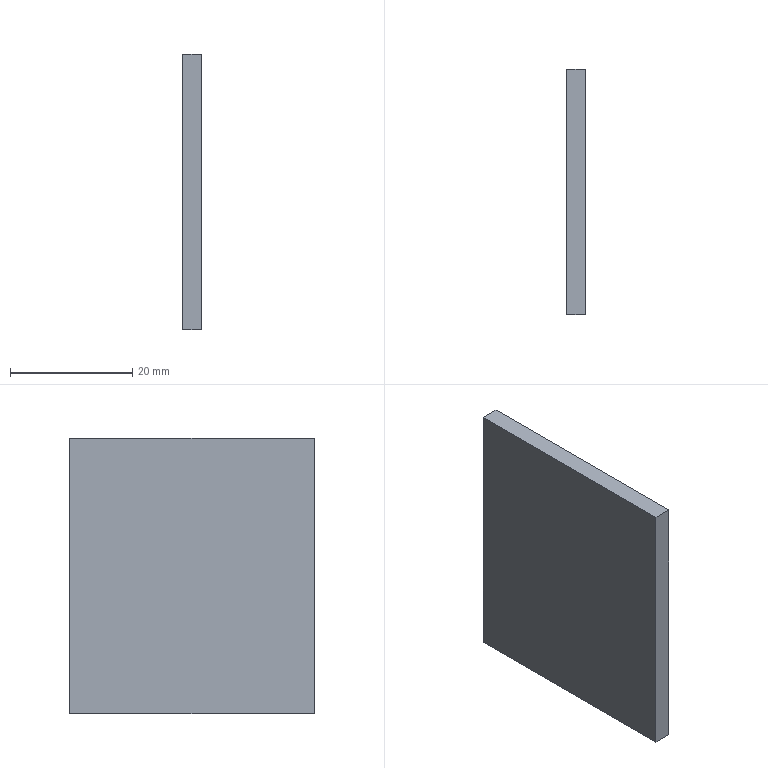Part | STEP file | Positioning_id1638_x_t | 1 solid | 6 faces | box 3 x 40 x 45 mm | volume 5400 mm3 | plane 6
STEP:
#1=CARTESIAN_POINT('',(0.,0.,0.));
#2=DIRECTION('',(0.,0.,1.));
#3=DIRECTION('',(1.,0.,0.));
#4=AXIS2_PLACEMENT_3D('',#1,#2,#3);
#5=CARTESIAN_POINT('',(-790.002,465.,51.995));
#6=VERTEX_POINT('',#5);
#7=CARTESIAN_POINT('',(-793.002,465.,51.995));
#8=VERTEX_POINT('',#7);
#9=CARTESIAN_POINT('',(-790.002,465.,51.995));
#10=DIRECTION('',(-1.,0.,0.));
#11=VECTOR('',#10,1.);
#12=LINE('',#9,#11);
#13=CARTESIAN_POINT('',(-762.002,465.,51.995));
#14=DIRECTION('',(0.,0.,-1.));
#15=DIRECTION('',(1.,0.,0.));
#16=AXIS2_PLACEMENT_3D('',#13,#14,#15);
#17=PLANE('',#16);
#18=CARTESIAN_POINT('',(-28.,0.));
#19=DIRECTION('',(-1.,0.));
#20=VECTOR('',#19,1.);
#21=LINE('',#18,#20);
#22=(GEOMETRIC_REPRESENTATION_CONTEXT(2)PARAMETRIC_REPRESENTATION_CONTEXT()REPRESENTATION_CONTEXT('',''));
#23=DEFINITIONAL_REPRESENTATION('',(#21),#22);
#24=PCURVE('',#17,#23);
#25=CARTESIAN_POINT('',(-828.002,465.,116.995));
#26=DIRECTION('',(0.,-1.,0.));
#27=DIRECTION('',(-1.,0.,0.));
#28=AXIS2_PLACEMENT_3D('',#25,#26,#27);
#29=PLANE('',#28);
#30=CARTESIAN_POINT('',(-38.,65.));
#31=DIRECTION('',(1.,0.));
#32=VECTOR('',#31,1.);
#33=LINE('',#30,#32);
#34=(GEOMETRIC_REPRESENTATION_CONTEXT(2)PARAMETRIC_REPRESENTATION_CONTEXT()REPRESENTATION_CONTEXT('',''));
#35=DEFINITIONAL_REPRESENTATION('',(#33),#34);
#36=PCURVE('',#29,#35);
#37=SURFACE_CURVE('',#12,(#24,#36),.PCURVE_S1.);
#38=EDGE_CURVE('',#6,#8,#37,.T.);
#39=ORIENTED_EDGE('',*,*,#38,.T.);
#40=CARTESIAN_POINT('',(-793.002,505.,51.995));
#41=VERTEX_POINT('',#40);
#42=CARTESIAN_POINT('',(-793.002,465.,51.995));
#43=DIRECTION('',(0.,1.,0.));
#44=VECTOR('',#43,1.);
#45=LINE('',#42,#44);
#46=CARTESIAN_POINT('',(-31.,0.));
#47=DIRECTION('',(0.,-1.));
#48=VECTOR('',#47,1.);
#49=LINE('',#46,#48);
#50=(GEOMETRIC_REPRESENTATION_CONTEXT(2)PARAMETRIC_REPRESENTATION_CONTEXT()REPRESENTATION_CONTEXT('',''));
#51=DEFINITIONAL_REPRESENTATION('',(#49),#50);
#52=PCURVE('',#17,#51);
#53=CARTESIAN_POINT('',(-793.002,495.,116.995));
#54=DIRECTION('',(-1.,0.,0.));
#55=DIRECTION('',(0.,0.,-1.));
#56=AXIS2_PLACEMENT_3D('',#53,#54,#55);
#57=PLANE('',#56);
#58=CARTESIAN_POINT('',(65.,30.));
#59=DIRECTION('',(0.,-1.));
#60=VECTOR('',#59,1.);
#61=LINE('',#58,#60);
#62=(GEOMETRIC_REPRESENTATION_CONTEXT(2)PARAMETRIC_REPRESENTATION_CONTEXT()REPRESENTATION_CONTEXT('',''));
#63=DEFINITIONAL_REPRESENTATION('',(#61),#62);
#64=PCURVE('',#57,#63);
#65=SURFACE_CURVE('',#45,(#52,#64),.PCURVE_S1.);
#66=EDGE_CURVE('',#8,#41,#65,.T.);
#67=ORIENTED_EDGE('',*,*,#66,.T.);
#68=CARTESIAN_POINT('',(-790.002,505.,51.995));
#69=VERTEX_POINT('',#68);
#70=CARTESIAN_POINT('',(-793.002,505.,51.995));
#71=DIRECTION('',(1.,0.,0.));
#72=VECTOR('',#71,1.);
#73=LINE('',#70,#72);
#74=CARTESIAN_POINT('',(-31.,-40.));
#75=DIRECTION('',(1.,0.));
#76=VECTOR('',#75,1.);
#77=LINE('',#74,#76);
#78=(GEOMETRIC_REPRESENTATION_CONTEXT(2)PARAMETRIC_REPRESENTATION_CONTEXT()REPRESENTATION_CONTEXT('',''));
#79=DEFINITIONAL_REPRESENTATION('',(#77),#78);
#80=PCURVE('',#17,#79);
#81=CARTESIAN_POINT('',(-828.002,505.,116.995));
#82=DIRECTION('',(0.,1.,0.));
#83=DIRECTION('',(1.,0.,0.));
#84=AXIS2_PLACEMENT_3D('',#81,#82,#83);
#85=PLANE('',#84);
#86=CARTESIAN_POINT('',(35.,65.));
#87=DIRECTION('',(1.,0.));
#88=VECTOR('',#87,1.);
#89=LINE('',#86,#88);
#90=(GEOMETRIC_REPRESENTATION_CONTEXT(2)PARAMETRIC_REPRESENTATION_CONTEXT()REPRESENTATION_CONTEXT('',''));
#91=DEFINITIONAL_REPRESENTATION('',(#89),#90);
#92=PCURVE('',#85,#91);
#93=SURFACE_CURVE('',#73,(#80,#92),.PCURVE_S1.);
#94=EDGE_CURVE('',#41,#69,#93,.T.);
#95=ORIENTED_EDGE('',*,*,#94,.T.);
#96=CARTESIAN_POINT('',(-790.002,465.,51.995));
#97=DIRECTION('',(0.,1.,0.));
#98=VECTOR('',#97,1.);
#99=LINE('',#96,#98);
#100=CARTESIAN_POINT('',(-28.,0.));
#101=DIRECTION('',(0.,-1.));
#102=VECTOR('',#101,1.);
#103=LINE('',#100,#102);
#104=(GEOMETRIC_REPRESENTATION_CONTEXT(2)PARAMETRIC_REPRESENTATION_CONTEXT()REPRESENTATION_CONTEXT('',''));
#105=DEFINITIONAL_REPRESENTATION('',(#103),#104);
#106=PCURVE('',#17,#105);
#107=CARTESIAN_POINT('',(-790.002,465.,96.995));
#108=DIRECTION('',(1.,0.,0.));
#109=DIRECTION('',(0.,0.,1.));
#110=AXIS2_PLACEMENT_3D('',#107,#108,#109);
#111=PLANE('',#110);
#112=CARTESIAN_POINT('',(-45.,0.));
#113=DIRECTION('',(0.,-1.));
#114=VECTOR('',#113,1.);
#115=LINE('',#112,#114);
#116=(GEOMETRIC_REPRESENTATION_CONTEXT(2)PARAMETRIC_REPRESENTATION_CONTEXT()REPRESENTATION_CONTEXT('',''));
#117=DEFINITIONAL_REPRESENTATION('',(#115),#116);
#118=PCURVE('',#111,#117);
#119=SURFACE_CURVE('',#99,(#106,#118),.PCURVE_S1.);
#120=EDGE_CURVE('',#6,#69,#119,.T.);
#121=ORIENTED_EDGE('',*,*,#120,.F.);
#122=EDGE_LOOP('',(#39,#67,#95,#121));
#123=FACE_BOUND('',#122,.T.);
#124=ADVANCED_FACE('',(#123),#17,.T.);
#125=CARTESIAN_POINT('',(-793.002,505.,96.995));
#126=VERTEX_POINT('',#125);
#127=CARTESIAN_POINT('',(-790.002,505.,96.995));
#128=VERTEX_POINT('',#127);
#129=CARTESIAN_POINT('',(-793.002,505.,96.995));
#130=DIRECTION('',(1.,0.,0.));
#131=VECTOR('',#130,1.);
#132=LINE('',#129,#131);
#133=CARTESIAN_POINT('',(-828.002,495.,96.995));
#134=DIRECTION('',(0.,0.,1.));
#135=DIRECTION('',(-1.,0.,0.));
#136=AXIS2_PLACEMENT_3D('',#133,#134,#135);
#137=PLANE('',#136);
#138=CARTESIAN_POINT('',(-35.,-10.));
#139=DIRECTION('',(-1.,0.));
#140=VECTOR('',#139,1.);
#141=LINE('',#138,#140);
#142=(GEOMETRIC_REPRESENTATION_CONTEXT(2)PARAMETRIC_REPRESENTATION_CONTEXT()REPRESENTATION_CONTEXT('',''));
#143=DEFINITIONAL_REPRESENTATION('',(#141),#142);
#144=PCURVE('',#137,#143);
#145=CARTESIAN_POINT('',(35.,20.));
#146=DIRECTION('',(1.,0.));
#147=VECTOR('',#146,1.);
#148=LINE('',#145,#147);
#149=(GEOMETRIC_REPRESENTATION_CONTEXT(2)PARAMETRIC_REPRESENTATION_CONTEXT()REPRESENTATION_CONTEXT('',''));
#150=DEFINITIONAL_REPRESENTATION('',(#148),#149);
#151=PCURVE('',#85,#150);
#152=SURFACE_CURVE('',#132,(#144,#151),.PCURVE_S1.);
#153=EDGE_CURVE('',#126,#128,#152,.T.);
#154=ORIENTED_EDGE('',*,*,#153,.F.);
#155=CARTESIAN_POINT('',(-793.002,465.,96.995));
#156=VERTEX_POINT('',#155);
#157=CARTESIAN_POINT('',(-793.002,465.,96.995));
#158=DIRECTION('',(0.,1.,0.));
#159=VECTOR('',#158,1.);
#160=LINE('',#157,#159);
#161=CARTESIAN_POINT('',(-35.,30.));
#162=DIRECTION('',(0.,-1.));
#163=VECTOR('',#162,1.);
#164=LINE('',#161,#163);
#165=(GEOMETRIC_REPRESENTATION_CONTEXT(2)PARAMETRIC_REPRESENTATION_CONTEXT()REPRESENTATION_CONTEXT('',''));
#166=DEFINITIONAL_REPRESENTATION('',(#164),#165);
#167=PCURVE('',#137,#166);
#168=CARTESIAN_POINT('',(20.,30.));
#169=DIRECTION('',(0.,-1.));
#170=VECTOR('',#169,1.);
#171=LINE('',#168,#170);
#172=(GEOMETRIC_REPRESENTATION_CONTEXT(2)PARAMETRIC_REPRESENTATION_CONTEXT()REPRESENTATION_CONTEXT('',''));
#173=DEFINITIONAL_REPRESENTATION('',(#171),#172);
#174=PCURVE('',#57,#173);
#175=SURFACE_CURVE('',#160,(#167,#174),.PCURVE_S1.);
#176=EDGE_CURVE('',#156,#126,#175,.T.);
#177=ORIENTED_EDGE('',*,*,#176,.F.);
#178=CARTESIAN_POINT('',(-790.002,465.,96.995));
#179=VERTEX_POINT('',#178);
#180=CARTESIAN_POINT('',(-793.002,465.,96.995));
#181=DIRECTION('',(1.,0.,0.));
#182=VECTOR('',#181,1.);
#183=LINE('',#180,#182);
#184=CARTESIAN_POINT('',(-35.,30.));
#185=DIRECTION('',(-1.,0.));
#186=VECTOR('',#185,1.);
#187=LINE('',#184,#186);
#188=(GEOMETRIC_REPRESENTATION_CONTEXT(2)PARAMETRIC_REPRESENTATION_CONTEXT()REPRESENTATION_CONTEXT('',''));
#189=DEFINITIONAL_REPRESENTATION('',(#187),#188);
#190=PCURVE('',#137,#189);
#191=CARTESIAN_POINT('',(-35.,20.));
#192=DIRECTION('',(-1.,0.));
#193=VECTOR('',#192,1.);
#194=LINE('',#191,#193);
#195=(GEOMETRIC_REPRESENTATION_CONTEXT(2)PARAMETRIC_REPRESENTATION_CONTEXT()REPRESENTATION_CONTEXT('',''));
#196=DEFINITIONAL_REPRESENTATION('',(#194),#195);
#197=PCURVE('',#29,#196);
#198=SURFACE_CURVE('',#183,(#190,#197),.PCURVE_S1.);
#199=EDGE_CURVE('',#156,#179,#198,.T.);
#200=ORIENTED_EDGE('',*,*,#199,.T.);
#201=CARTESIAN_POINT('',(-790.002,505.,96.995));
#202=DIRECTION('',(0.,-1.,0.));
#203=VECTOR('',#202,1.);
#204=LINE('',#201,#203);
#205=CARTESIAN_POINT('',(-38.,-10.));
#206=DIRECTION('',(0.,1.));
#207=VECTOR('',#206,1.);
#208=LINE('',#205,#207);
#209=(GEOMETRIC_REPRESENTATION_CONTEXT(2)PARAMETRIC_REPRESENTATION_CONTEXT()REPRESENTATION_CONTEXT('',''));
#210=DEFINITIONAL_REPRESENTATION('',(#208),#209);
#211=PCURVE('',#137,#210);
#212=CARTESIAN_POINT('',(0.,-40.));
#213=DIRECTION('',(0.,1.));
#214=VECTOR('',#213,1.);
#215=LINE('',#212,#214);
#216=(GEOMETRIC_REPRESENTATION_CONTEXT(2)PARAMETRIC_REPRESENTATION_CONTEXT()REPRESENTATION_CONTEXT('',''));
#217=DEFINITIONAL_REPRESENTATION('',(#215),#216);
#218=PCURVE('',#111,#217);
#219=SURFACE_CURVE('',#204,(#211,#218),.PCURVE_S1.);
#220=EDGE_CURVE('',#128,#179,#219,.T.);
#221=ORIENTED_EDGE('',*,*,#220,.F.);
#222=EDGE_LOOP('',(#154,#177,#200,#221));
#223=FACE_BOUND('',#222,.T.);
#224=ADVANCED_FACE('',(#223),#137,.T.);
#225=ORIENTED_EDGE('',*,*,#94,.F.);
#226=CARTESIAN_POINT('',(-793.002,505.,96.995));
#227=DIRECTION('',(0.,0.,-1.));
#228=VECTOR('',#227,1.);
#229=LINE('',#226,#228);
#230=CARTESIAN_POINT('',(35.,20.));
#231=DIRECTION('',(0.,1.));
#232=VECTOR('',#231,1.);
#233=LINE('',#230,#232);
#234=(GEOMETRIC_REPRESENTATION_CONTEXT(2)PARAMETRIC_REPRESENTATION_CONTEXT()REPRESENTATION_CONTEXT('',''));
#235=DEFINITIONAL_REPRESENTATION('',(#233),#234);
#236=PCURVE('',#85,#235);
#237=CARTESIAN_POINT('',(20.,-10.));
#238=DIRECTION('',(1.,0.));
#239=VECTOR('',#238,1.);
#240=LINE('',#237,#239);
#241=(GEOMETRIC_REPRESENTATION_CONTEXT(2)PARAMETRIC_REPRESENTATION_CONTEXT()REPRESENTATION_CONTEXT('',''));
#242=DEFINITIONAL_REPRESENTATION('',(#240),#241);
#243=PCURVE('',#57,#242);
#244=SURFACE_CURVE('',#229,(#236,#243),.PCURVE_S1.);
#245=EDGE_CURVE('',#126,#41,#244,.T.);
#246=ORIENTED_EDGE('',*,*,#245,.F.);
#247=ORIENTED_EDGE('',*,*,#153,.T.);
#248=CARTESIAN_POINT('',(-790.002,505.,51.995));
#249=DIRECTION('',(0.,0.,1.));
#250=VECTOR('',#249,1.);
#251=LINE('',#248,#250);
#252=CARTESIAN_POINT('',(38.,65.));
#253=DIRECTION('',(0.,-1.));
#254=VECTOR('',#253,1.);
#255=LINE('',#252,#254);
#256=(GEOMETRIC_REPRESENTATION_CONTEXT(2)PARAMETRIC_REPRESENTATION_CONTEXT()REPRESENTATION_CONTEXT('',''));
#257=DEFINITIONAL_REPRESENTATION('',(#255),#256);
#258=PCURVE('',#85,#257);
#259=CARTESIAN_POINT('',(-45.,-40.));
#260=DIRECTION('',(1.,0.));
#261=VECTOR('',#260,1.);
#262=LINE('',#259,#261);
#263=(GEOMETRIC_REPRESENTATION_CONTEXT(2)PARAMETRIC_REPRESENTATION_CONTEXT()REPRESENTATION_CONTEXT('',''));
#264=DEFINITIONAL_REPRESENTATION('',(#262),#263);
#265=PCURVE('',#111,#264);
#266=SURFACE_CURVE('',#251,(#258,#265),.PCURVE_S1.);
#267=EDGE_CURVE('',#69,#128,#266,.T.);
#268=ORIENTED_EDGE('',*,*,#267,.F.);
#269=EDGE_LOOP('',(#225,#246,#247,#268));
#270=FACE_BOUND('',#269,.T.);
#271=ADVANCED_FACE('',(#270),#85,.T.);
#272=ORIENTED_EDGE('',*,*,#199,.F.);
#273=CARTESIAN_POINT('',(-793.002,465.,51.995));
#274=DIRECTION('',(0.,0.,1.));
#275=VECTOR('',#274,1.);
#276=LINE('',#273,#275);
#277=CARTESIAN_POINT('',(-35.,65.));
#278=DIRECTION('',(0.,-1.));
#279=VECTOR('',#278,1.);
#280=LINE('',#277,#279);
#281=(GEOMETRIC_REPRESENTATION_CONTEXT(2)PARAMETRIC_REPRESENTATION_CONTEXT()REPRESENTATION_CONTEXT('',''));
#282=DEFINITIONAL_REPRESENTATION('',(#280),#281);
#283=PCURVE('',#29,#282);
#284=CARTESIAN_POINT('',(65.,30.));
#285=DIRECTION('',(-1.,0.));
#286=VECTOR('',#285,1.);
#287=LINE('',#284,#286);
#288=(GEOMETRIC_REPRESENTATION_CONTEXT(2)PARAMETRIC_REPRESENTATION_CONTEXT()REPRESENTATION_CONTEXT('',''));
#289=DEFINITIONAL_REPRESENTATION('',(#287),#288);
#290=PCURVE('',#57,#289);
#291=SURFACE_CURVE('',#276,(#283,#290),.PCURVE_S1.);
#292=EDGE_CURVE('',#8,#156,#291,.T.);
#293=ORIENTED_EDGE('',*,*,#292,.F.);
#294=ORIENTED_EDGE('',*,*,#38,.F.);
#295=CARTESIAN_POINT('',(-790.002,465.,96.995));
#296=DIRECTION('',(0.,0.,-1.));
#297=VECTOR('',#296,1.);
#298=LINE('',#295,#297);
#299=CARTESIAN_POINT('',(-38.,20.));
#300=DIRECTION('',(0.,1.));
#301=VECTOR('',#300,1.);
#302=LINE('',#299,#301);
#303=(GEOMETRIC_REPRESENTATION_CONTEXT(2)PARAMETRIC_REPRESENTATION_CONTEXT()REPRESENTATION_CONTEXT('',''));
#304=DEFINITIONAL_REPRESENTATION('',(#302),#303);
#305=PCURVE('',#29,#304);
#306=CARTESIAN_POINT('',(0.,0.));
#307=DIRECTION('',(-1.,0.));
#308=VECTOR('',#307,1.);
#309=LINE('',#306,#308);
#310=(GEOMETRIC_REPRESENTATION_CONTEXT(2)PARAMETRIC_REPRESENTATION_CONTEXT()REPRESENTATION_CONTEXT('',''));
#311=DEFINITIONAL_REPRESENTATION('',(#309),#310);
#312=PCURVE('',#111,#311);
#313=SURFACE_CURVE('',#298,(#305,#312),.PCURVE_S1.);
#314=EDGE_CURVE('',#179,#6,#313,.T.);
#315=ORIENTED_EDGE('',*,*,#314,.F.);
#316=EDGE_LOOP('',(#272,#293,#294,#315));
#317=FACE_BOUND('',#316,.T.);
#318=ADVANCED_FACE('',(#317),#29,.T.);
#319=ORIENTED_EDGE('',*,*,#292,.T.);
#320=ORIENTED_EDGE('',*,*,#176,.T.);
#321=ORIENTED_EDGE('',*,*,#245,.T.);
#322=ORIENTED_EDGE('',*,*,#66,.F.);
#323=EDGE_LOOP('',(#319,#320,#321,#322));
#324=FACE_BOUND('',#323,.T.);
#325=ADVANCED_FACE('',(#324),#57,.T.);
#326=ORIENTED_EDGE('',*,*,#267,.T.);
#327=ORIENTED_EDGE('',*,*,#220,.T.);
#328=ORIENTED_EDGE('',*,*,#314,.T.);
#329=ORIENTED_EDGE('',*,*,#120,.T.);
#330=EDGE_LOOP('',(#326,#327,#328,#329));
#331=FACE_BOUND('',#330,.T.);
#332=ADVANCED_FACE('',(#331),#111,.T.);
#333=CLOSED_SHELL('',(#124,#224,#271,#318,#325,#332));
#334=MANIFOLD_SOLID_BREP('',#333);
#335=(LENGTH_UNIT()NAMED_UNIT(*)SI_UNIT(.MILLI.,.METRE.));
#336=UNCERTAINTY_MEASURE_WITH_UNIT(LENGTH_MEASURE(0.0000001),#335,'','');
#337=(NAMED_UNIT(*)PLANE_ANGLE_UNIT()SI_UNIT($,.RADIAN.));
#338=(NAMED_UNIT(*)SI_UNIT($,.STERADIAN.)SOLID_ANGLE_UNIT());
#339=(GEOMETRIC_REPRESENTATION_CONTEXT(3)GLOBAL_UNCERTAINTY_ASSIGNED_CONTEXT((#336))GLOBAL_UNIT_ASSIGNED_CONTEXT((#335,#337,#338))REPRESENTATION_CONTEXT('',''));
#340=ADVANCED_BREP_SHAPE_REPRESENTATION('',(#4,#334),#339);